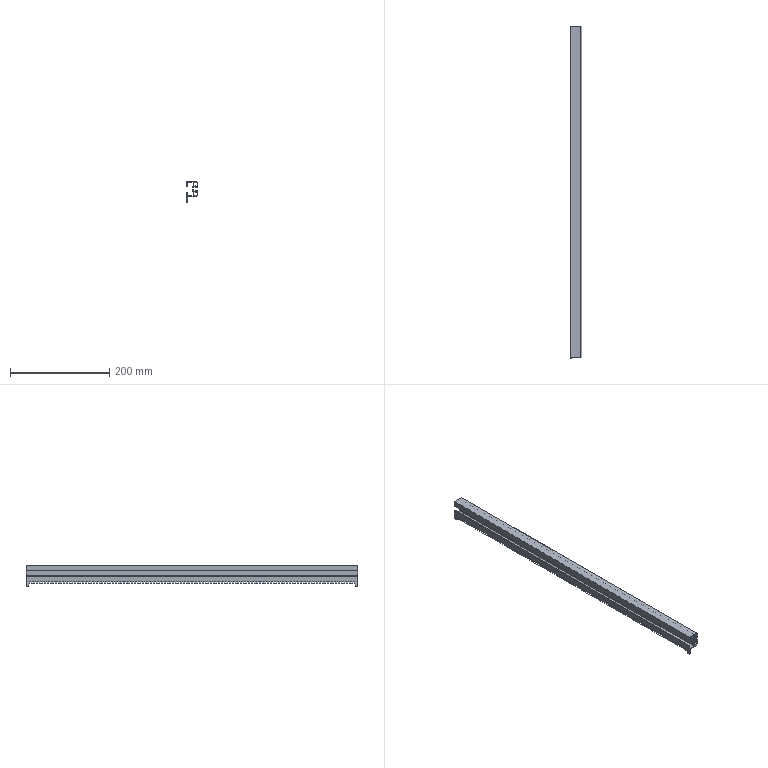Part | STEP file | DEWALT-DWE7492-B22 | 1 solid | 542 faces | box 24 x 670 x 42.688 mm | volume 151895 mm3 | plane 522 | cylinder 20 | commonest cylinder face diameters 1 x16 3.8 x4